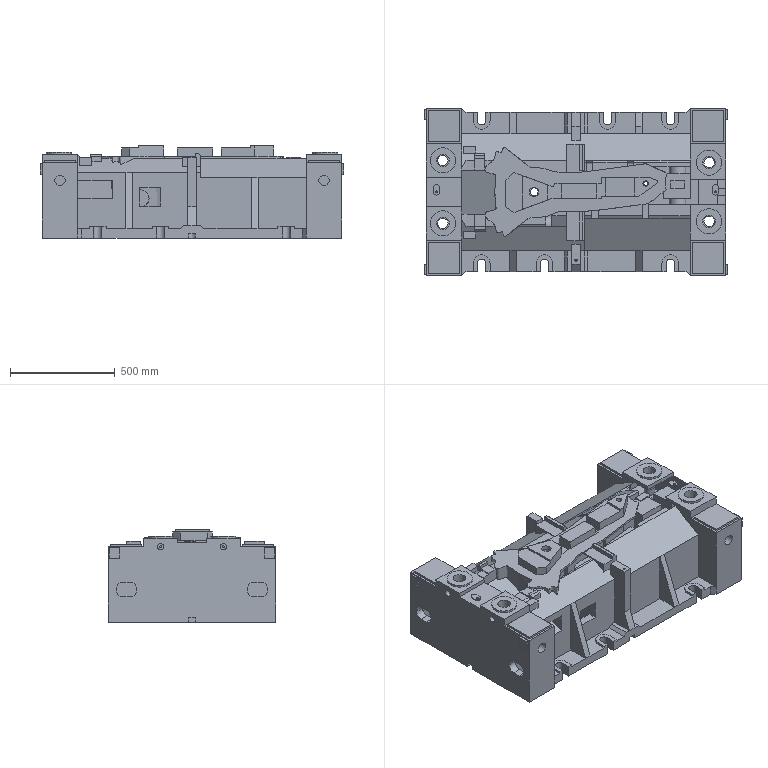Part | NX | features solid 2 | 1 solid | 580 faces | box 1450 x 800 x 440 mm | volume 184592094 mm3 | plane 473 | cylinder 87 | spline 20 | commonest cylinder face diameters 80 x22 60 x20 10 x8 30 x8 50 x8 40 x6